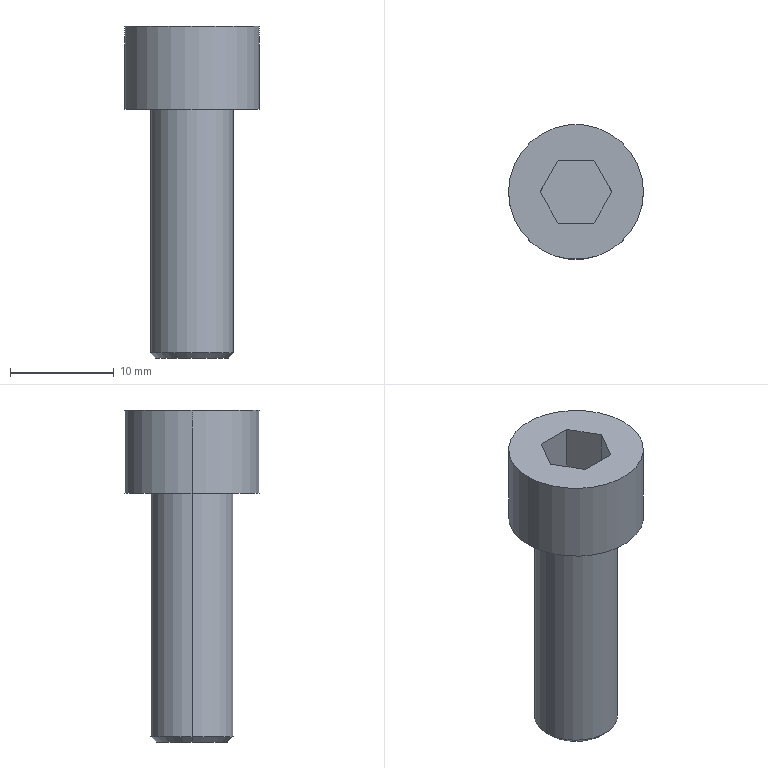Part | Creo | 1 solid | 16 faces | box 13 x 13 x 32 mm | volume 2101 mm3 | plane 10 | cylinder 4 | cone 2 | commonest cylinder face diameters 8 x2 13 x2
STEP:
#1=CARTESIAN_POINT('',(0.,0.,0.));
#2=DIRECTION('',(0.,0.,1.));
#3=DIRECTION('',(1.,0.,0.));
#4=AXIS2_PLACEMENT_3D('',#1,#2,#3);
#5=CARTESIAN_POINT('',(382.148,-184.728,-64.336));
#6=VERTEX_POINT('',#5);
#7=CARTESIAN_POINT('',(390.148,-184.728,-64.336));
#8=VERTEX_POINT('',#7);
#9=CARTESIAN_POINT('',(386.148,-184.728,-64.336));
#10=DIRECTION('',(0.,0.,-1.));
#11=DIRECTION('',(-1.,0.,0.));
#12=AXIS2_PLACEMENT_3D('',#9,#10,#11);
#13=CIRCLE('',#12,4.);
#14=EDGE_CURVE('',#6,#8,#13,.T.);
#15=ORIENTED_EDGE('',*,*,#14,.T.);
#16=CARTESIAN_POINT('',(390.148,-184.728,-40.844));
#17=VERTEX_POINT('',#16);
#18=CARTESIAN_POINT('',(390.148,-184.728,-40.844));
#19=DIRECTION('',(0.,0.,-1.));
#20=VECTOR('',#19,23.493);
#21=LINE('',#18,#20);
#22=EDGE_CURVE('',#17,#8,#21,.T.);
#23=ORIENTED_EDGE('',*,*,#22,.F.);
#24=CARTESIAN_POINT('',(382.148,-184.728,-40.844));
#25=VERTEX_POINT('',#24);
#26=CARTESIAN_POINT('',(386.148,-184.728,-40.844));
#27=DIRECTION('',(0.,0.,1.));
#28=DIRECTION('',(1.,0.,0.));
#29=AXIS2_PLACEMENT_3D('',#26,#27,#28);
#30=CIRCLE('',#29,4.);
#31=EDGE_CURVE('',#17,#25,#30,.T.);
#32=ORIENTED_EDGE('',*,*,#31,.T.);
#33=CARTESIAN_POINT('',(382.148,-184.728,-40.844));
#34=DIRECTION('',(0.,0.,-1.));
#35=VECTOR('',#34,23.493);
#36=LINE('',#33,#35);
#37=EDGE_CURVE('',#25,#6,#36,.T.);
#38=ORIENTED_EDGE('',*,*,#37,.T.);
#39=EDGE_LOOP('',(#15,#23,#32,#38));
#40=FACE_OUTER_BOUND('',#39,.F.);
#41=CARTESIAN_POINT('',(386.148,-184.728,-40.844));
#42=DIRECTION('',(0.,0.,-1.));
#43=DIRECTION('',(-1.,0.,0.));
#44=AXIS2_PLACEMENT_3D('',#41,#42,#43);
#45=CYLINDRICAL_SURFACE('',#44,4.);
#46=ADVANCED_FACE('',(#40),#45,.T.);
#47=CARTESIAN_POINT('',(382.656,-184.728,-64.844));
#48=VERTEX_POINT('',#47);
#49=CARTESIAN_POINT('',(389.641,-184.728,-64.844));
#50=VERTEX_POINT('',#49);
#51=CARTESIAN_POINT('',(386.148,-184.728,-64.844));
#52=DIRECTION('',(0.,0.,-1.));
#53=DIRECTION('',(-1.,0.,0.));
#54=AXIS2_PLACEMENT_3D('',#51,#52,#53);
#55=CIRCLE('',#54,3.493);
#56=EDGE_CURVE('',#48,#50,#55,.T.);
#57=ORIENTED_EDGE('',*,*,#56,.T.);
#58=CARTESIAN_POINT('',(389.641,-184.728,-64.844));
#59=DIRECTION('',(0.7071,0.,0.7071));
#60=VECTOR('',#59,0.7176);
#61=LINE('',#58,#60);
#62=EDGE_CURVE('',#50,#8,#61,.T.);
#63=ORIENTED_EDGE('',*,*,#62,.T.);
#64=ORIENTED_EDGE('',*,*,#14,.F.);
#65=CARTESIAN_POINT('',(382.656,-184.728,-64.844));
#66=DIRECTION('',(-0.7071,0.,0.7071));
#67=VECTOR('',#66,0.7176);
#68=LINE('',#65,#67);
#69=EDGE_CURVE('',#48,#6,#68,.T.);
#70=ORIENTED_EDGE('',*,*,#69,.F.);
#71=EDGE_LOOP('',(#57,#63,#64,#70));
#72=FACE_OUTER_BOUND('',#71,.F.);
#73=CARTESIAN_POINT('',(386.148,-184.728,-64.59));
#74=DIRECTION('',(0.,0.,1.));
#75=DIRECTION('',(1.,0.,0.));
#76=AXIS2_PLACEMENT_3D('',#73,#74,#75);
#77=CONICAL_SURFACE('',#76,3.746,45.);
#78=ADVANCED_FACE('',(#72),#77,.T.);
#79=ORIENTED_EDGE('',*,*,#56,.F.);
#80=CARTESIAN_POINT('',(386.148,-184.728,-64.844));
#81=DIRECTION('',(0.,0.,-1.));
#82=DIRECTION('',(1.,0.,0.));
#83=AXIS2_PLACEMENT_3D('',#80,#81,#82);
#84=CIRCLE('',#83,3.493);
#85=EDGE_CURVE('',#50,#48,#84,.T.);
#86=ORIENTED_EDGE('',*,*,#85,.F.);
#87=EDGE_LOOP('',(#79,#86));
#88=FACE_OUTER_BOUND('',#87,.F.);
#89=CARTESIAN_POINT('',(386.148,-184.728,-64.844));
#90=DIRECTION('',(0.,0.,1.));
#91=DIRECTION('',(1.,0.,0.));
#92=AXIS2_PLACEMENT_3D('',#89,#90,#91);
#93=PLANE('',#92);
#94=ADVANCED_FACE('',(#88),#93,.F.);
#95=ORIENTED_EDGE('',*,*,#85,.T.);
#96=ORIENTED_EDGE('',*,*,#69,.T.);
#97=CARTESIAN_POINT('',(386.148,-184.728,-64.336));
#98=DIRECTION('',(0.,0.,-1.));
#99=DIRECTION('',(1.,0.,0.));
#100=AXIS2_PLACEMENT_3D('',#97,#98,#99);
#101=CIRCLE('',#100,4.);
#102=EDGE_CURVE('',#8,#6,#101,.T.);
#103=ORIENTED_EDGE('',*,*,#102,.F.);
#104=ORIENTED_EDGE('',*,*,#62,.F.);
#105=EDGE_LOOP('',(#95,#96,#103,#104));
#106=FACE_OUTER_BOUND('',#105,.F.);
#107=CARTESIAN_POINT('',(386.148,-184.728,-64.59));
#108=DIRECTION('',(0.,0.,1.));
#109=DIRECTION('',(1.,0.,0.));
#110=AXIS2_PLACEMENT_3D('',#107,#108,#109);
#111=CONICAL_SURFACE('',#110,3.746,45.);
#112=ADVANCED_FACE('',(#106),#111,.T.);
#113=ORIENTED_EDGE('',*,*,#102,.T.);
#114=ORIENTED_EDGE('',*,*,#37,.F.);
#115=CARTESIAN_POINT('',(386.148,-184.728,-40.844));
#116=DIRECTION('',(0.,0.,1.));
#117=DIRECTION('',(-1.,0.,0.));
#118=AXIS2_PLACEMENT_3D('',#115,#116,#117);
#119=CIRCLE('',#118,4.);
#120=EDGE_CURVE('',#25,#17,#119,.T.);
#121=ORIENTED_EDGE('',*,*,#120,.T.);
#122=ORIENTED_EDGE('',*,*,#22,.T.);
#123=EDGE_LOOP('',(#113,#114,#121,#122));
#124=FACE_OUTER_BOUND('',#123,.F.);
#125=CARTESIAN_POINT('',(386.148,-184.728,-40.844));
#126=DIRECTION('',(0.,0.,-1.));
#127=DIRECTION('',(-1.,0.,0.));
#128=AXIS2_PLACEMENT_3D('',#125,#126,#127);
#129=CYLINDRICAL_SURFACE('',#128,4.);
#130=ADVANCED_FACE('',(#124),#129,.T.);
#131=CARTESIAN_POINT('',(379.648,-184.728,-40.844));
#132=VERTEX_POINT('',#131);
#133=CARTESIAN_POINT('',(392.648,-184.728,-40.844));
#134=VERTEX_POINT('',#133);
#135=CARTESIAN_POINT('',(386.148,-184.728,-40.844));
#136=DIRECTION('',(0.,0.,-1.));
#137=DIRECTION('',(-1.,0.,0.));
#138=AXIS2_PLACEMENT_3D('',#135,#136,#137);
#139=CIRCLE('',#138,6.5);
#140=EDGE_CURVE('',#132,#134,#139,.T.);
#141=ORIENTED_EDGE('',*,*,#140,.F.);
#142=CARTESIAN_POINT('',(386.148,-184.728,-40.844));
#143=DIRECTION('',(0.,0.,-1.));
#144=DIRECTION('',(1.,0.,0.));
#145=AXIS2_PLACEMENT_3D('',#142,#143,#144);
#146=CIRCLE('',#145,6.5);
#147=EDGE_CURVE('',#134,#132,#146,.T.);
#148=ORIENTED_EDGE('',*,*,#147,.F.);
#149=EDGE_LOOP('',(#141,#148));
#150=FACE_OUTER_BOUND('',#149,.F.);
#151=ORIENTED_EDGE('',*,*,#120,.F.);
#152=ORIENTED_EDGE('',*,*,#31,.F.);
#153=EDGE_LOOP('',(#151,#152));
#154=FACE_BOUND('',#153,.F.);
#155=CARTESIAN_POINT('',(386.148,-184.728,-40.844));
#156=DIRECTION('',(0.,0.,-1.));
#157=DIRECTION('',(-1.,0.,0.));
#158=AXIS2_PLACEMENT_3D('',#155,#156,#157);
#159=PLANE('',#158);
#160=ADVANCED_FACE('',(#150,#154),#159,.T.);
#161=CARTESIAN_POINT('',(392.648,-184.728,-32.844));
#162=VERTEX_POINT('',#161);
#163=CARTESIAN_POINT('',(379.648,-184.728,-32.844));
#164=VERTEX_POINT('',#163);
#165=CARTESIAN_POINT('',(386.148,-184.728,-32.844));
#166=DIRECTION('',(0.,0.,1.));
#167=DIRECTION('',(1.,0.,0.));
#168=AXIS2_PLACEMENT_3D('',#165,#166,#167);
#169=CIRCLE('',#168,6.5);
#170=EDGE_CURVE('',#162,#164,#169,.T.);
#171=ORIENTED_EDGE('',*,*,#170,.T.);
#172=CARTESIAN_POINT('',(379.648,-184.728,-40.844));
#173=DIRECTION('',(0.,0.,1.));
#174=VECTOR('',#173,8.);
#175=LINE('',#172,#174);
#176=EDGE_CURVE('',#132,#164,#175,.T.);
#177=ORIENTED_EDGE('',*,*,#176,.F.);
#178=ORIENTED_EDGE('',*,*,#140,.T.);
#179=CARTESIAN_POINT('',(392.648,-184.728,-40.844));
#180=DIRECTION('',(0.,0.,1.));
#181=VECTOR('',#180,8.);
#182=LINE('',#179,#181);
#183=EDGE_CURVE('',#134,#162,#182,.T.);
#184=ORIENTED_EDGE('',*,*,#183,.T.);
#185=EDGE_LOOP('',(#171,#177,#178,#184));
#186=FACE_OUTER_BOUND('',#185,.F.);
#187=CARTESIAN_POINT('',(386.148,-184.728,-40.844));
#188=DIRECTION('',(0.,0.,1.));
#189=DIRECTION('',(1.,0.,0.));
#190=AXIS2_PLACEMENT_3D('',#187,#188,#189);
#191=CYLINDRICAL_SURFACE('',#190,6.5);
#192=ADVANCED_FACE('',(#186),#191,.T.);
#193=CARTESIAN_POINT('',(386.148,-184.728,-32.844));
#194=DIRECTION('',(0.,0.,1.));
#195=DIRECTION('',(-1.,0.,0.));
#196=AXIS2_PLACEMENT_3D('',#193,#194,#195);
#197=CIRCLE('',#196,6.5);
#198=EDGE_CURVE('',#164,#162,#197,.T.);
#199=ORIENTED_EDGE('',*,*,#198,.F.);
#200=ORIENTED_EDGE('',*,*,#170,.F.);
#201=EDGE_LOOP('',(#199,#200));
#202=FACE_OUTER_BOUND('',#201,.F.);
#203=CARTESIAN_POINT('',(384.416,-181.728,-32.844));
#204=VERTEX_POINT('',#203);
#205=CARTESIAN_POINT('',(387.88,-181.728,-32.844));
#206=VERTEX_POINT('',#205);
#207=CARTESIAN_POINT('',(384.416,-181.728,-32.844));
#208=DIRECTION('',(1.,0.,0.));
#209=VECTOR('',#208,3.464);
#210=LINE('',#207,#209);
#211=EDGE_CURVE('',#204,#206,#210,.T.);
#212=ORIENTED_EDGE('',*,*,#211,.F.);
#213=CARTESIAN_POINT('',(382.684,-184.728,-32.844));
#214=VERTEX_POINT('',#213);
#215=CARTESIAN_POINT('',(382.684,-184.728,-32.844));
#216=DIRECTION('',(0.5,0.866,0.));
#217=VECTOR('',#216,3.464);
#218=LINE('',#215,#217);
#219=EDGE_CURVE('',#214,#204,#218,.T.);
#220=ORIENTED_EDGE('',*,*,#219,.F.);
#221=CARTESIAN_POINT('',(384.416,-187.728,-32.844));
#222=VERTEX_POINT('',#221);
#223=CARTESIAN_POINT('',(384.416,-187.728,-32.844));
#224=DIRECTION('',(-0.5,0.866,0.));
#225=VECTOR('',#224,3.464);
#226=LINE('',#223,#225);
#227=EDGE_CURVE('',#222,#214,#226,.T.);
#228=ORIENTED_EDGE('',*,*,#227,.F.);
#229=CARTESIAN_POINT('',(387.88,-187.728,-32.844));
#230=VERTEX_POINT('',#229);
#231=CARTESIAN_POINT('',(387.88,-187.728,-32.844));
#232=DIRECTION('',(-1.,0.,0.));
#233=VECTOR('',#232,3.464);
#234=LINE('',#231,#233);
#235=EDGE_CURVE('',#230,#222,#234,.T.);
#236=ORIENTED_EDGE('',*,*,#235,.F.);
#237=CARTESIAN_POINT('',(389.612,-184.728,-32.844));
#238=VERTEX_POINT('',#237);
#239=CARTESIAN_POINT('',(389.612,-184.728,-32.844));
#240=DIRECTION('',(-0.5,-0.866,0.));
#241=VECTOR('',#240,3.464);
#242=LINE('',#239,#241);
#243=EDGE_CURVE('',#238,#230,#242,.T.);
#244=ORIENTED_EDGE('',*,*,#243,.F.);
#245=CARTESIAN_POINT('',(387.88,-181.728,-32.844));
#246=DIRECTION('',(0.5,-0.866,0.));
#247=VECTOR('',#246,3.464);
#248=LINE('',#245,#247);
#249=EDGE_CURVE('',#206,#238,#248,.T.);
#250=ORIENTED_EDGE('',*,*,#249,.F.);
#251=EDGE_LOOP('',(#212,#220,#228,#236,#244,#250));
#252=FACE_BOUND('',#251,.F.);
#253=CARTESIAN_POINT('',(386.148,-184.728,-32.844));
#254=DIRECTION('',(0.,0.,1.));
#255=DIRECTION('',(1.,0.,0.));
#256=AXIS2_PLACEMENT_3D('',#253,#254,#255);
#257=PLANE('',#256);
#258=ADVANCED_FACE('',(#202,#252),#257,.T.);
#259=ORIENTED_EDGE('',*,*,#211,.T.);
#260=CARTESIAN_POINT('',(387.88,-181.728,-38.124));
#261=VERTEX_POINT('',#260);
#262=CARTESIAN_POINT('',(387.88,-181.728,-32.844));
#263=DIRECTION('',(0.,0.,-1.));
#264=VECTOR('',#263,5.28);
#265=LINE('',#262,#264);
#266=EDGE_CURVE('',#206,#261,#265,.T.);
#267=ORIENTED_EDGE('',*,*,#266,.T.);
#268=CARTESIAN_POINT('',(384.416,-181.728,-38.124));
#269=VERTEX_POINT('',#268);
#270=CARTESIAN_POINT('',(384.416,-181.728,-38.124));
#271=DIRECTION('',(1.,0.,0.));
#272=VECTOR('',#271,3.464);
#273=LINE('',#270,#272);
#274=EDGE_CURVE('',#269,#261,#273,.T.);
#275=ORIENTED_EDGE('',*,*,#274,.F.);
#276=CARTESIAN_POINT('',(384.416,-181.728,-32.844));
#277=DIRECTION('',(0.,0.,-1.));
#278=VECTOR('',#277,5.28);
#279=LINE('',#276,#278);
#280=EDGE_CURVE('',#204,#269,#279,.T.);
#281=ORIENTED_EDGE('',*,*,#280,.F.);
#282=EDGE_LOOP('',(#259,#267,#275,#281));
#283=FACE_OUTER_BOUND('',#282,.F.);
#284=CARTESIAN_POINT('',(387.88,-181.728,-38.124));
#285=DIRECTION('',(0.,1.,0.));
#286=DIRECTION('',(0.,0.,1.));
#287=AXIS2_PLACEMENT_3D('',#284,#285,#286);
#288=PLANE('',#287);
#289=ADVANCED_FACE('',(#283),#288,.F.);
#290=ORIENTED_EDGE('',*,*,#249,.T.);
#291=CARTESIAN_POINT('',(389.612,-184.728,-38.124));
#292=VERTEX_POINT('',#291);
#293=CARTESIAN_POINT('',(389.612,-184.728,-32.844));
#294=DIRECTION('',(0.,0.,-1.));
#295=VECTOR('',#294,5.28);
#296=LINE('',#293,#295);
#297=EDGE_CURVE('',#238,#292,#296,.T.);
#298=ORIENTED_EDGE('',*,*,#297,.T.);
#299=CARTESIAN_POINT('',(389.612,-184.728,-38.124));
#300=DIRECTION('',(-0.5,0.866,0.));
#301=VECTOR('',#300,3.464);
#302=LINE('',#299,#301);
#303=EDGE_CURVE('',#292,#261,#302,.T.);
#304=ORIENTED_EDGE('',*,*,#303,.T.);
#305=ORIENTED_EDGE('',*,*,#266,.F.);
#306=EDGE_LOOP('',(#290,#298,#304,#305));
#307=FACE_OUTER_BOUND('',#306,.F.);
#308=CARTESIAN_POINT('',(389.612,-184.728,-38.124));
#309=DIRECTION('',(0.866,0.5,0.));
#310=DIRECTION('',(-0.5,0.866,0.));
#311=AXIS2_PLACEMENT_3D('',#308,#309,#310);
#312=PLANE('',#311);
#313=ADVANCED_FACE('',(#307),#312,.F.);
#314=ORIENTED_EDGE('',*,*,#243,.T.);
#315=CARTESIAN_POINT('',(387.88,-187.728,-38.124));
#316=VERTEX_POINT('',#315);
#317=CARTESIAN_POINT('',(387.88,-187.728,-32.844));
#318=DIRECTION('',(0.,0.,-1.));
#319=VECTOR('',#318,5.28);
#320=LINE('',#317,#319);
#321=EDGE_CURVE('',#230,#316,#320,.T.);
#322=ORIENTED_EDGE('',*,*,#321,.T.);
#323=CARTESIAN_POINT('',(387.88,-187.728,-38.124));
#324=DIRECTION('',(0.5,0.866,0.));
#325=VECTOR('',#324,3.464);
#326=LINE('',#323,#325);
#327=EDGE_CURVE('',#316,#292,#326,.T.);
#328=ORIENTED_EDGE('',*,*,#327,.T.);
#329=ORIENTED_EDGE('',*,*,#297,.F.);
#330=EDGE_LOOP('',(#314,#322,#328,#329));
#331=FACE_OUTER_BOUND('',#330,.F.);
#332=CARTESIAN_POINT('',(387.88,-187.728,-38.124));
#333=DIRECTION('',(0.866,-0.5,0.));
#334=DIRECTION('',(0.5,0.866,0.));
#335=AXIS2_PLACEMENT_3D('',#332,#333,#334);
#336=PLANE('',#335);
#337=ADVANCED_FACE('',(#331),#336,.F.);
#338=ORIENTED_EDGE('',*,*,#235,.T.);
#339=CARTESIAN_POINT('',(384.416,-187.728,-38.124));
#340=VERTEX_POINT('',#339);
#341=CARTESIAN_POINT('',(384.416,-187.728,-32.844));
#342=DIRECTION('',(0.,0.,-1.));
#343=VECTOR('',#342,5.28);
#344=LINE('',#341,#343);
#345=EDGE_CURVE('',#222,#340,#344,.T.);
#346=ORIENTED_EDGE('',*,*,#345,.T.);
#347=CARTESIAN_POINT('',(387.88,-187.728,-38.124));
#348=DIRECTION('',(-1.,0.,0.));
#349=VECTOR('',#348,3.464);
#350=LINE('',#347,#349);
#351=EDGE_CURVE('',#316,#340,#350,.T.);
#352=ORIENTED_EDGE('',*,*,#351,.F.);
#353=ORIENTED_EDGE('',*,*,#321,.F.);
#354=EDGE_LOOP('',(#338,#346,#352,#353));
#355=FACE_OUTER_BOUND('',#354,.F.);
#356=CARTESIAN_POINT('',(384.416,-187.728,-38.124));
#357=DIRECTION('',(0.,-1.,0.));
#358=DIRECTION('',(0.,0.,-1.));
#359=AXIS2_PLACEMENT_3D('',#356,#357,#358);
#360=PLANE('',#359);
#361=ADVANCED_FACE('',(#355),#360,.F.);
#362=ORIENTED_EDGE('',*,*,#227,.T.);
#363=CARTESIAN_POINT('',(382.684,-184.728,-38.124));
#364=VERTEX_POINT('',#363);
#365=CARTESIAN_POINT('',(382.684,-184.728,-32.844));
#366=DIRECTION('',(0.,0.,-1.));
#367=VECTOR('',#366,5.28);
#368=LINE('',#365,#367);
#369=EDGE_CURVE('',#214,#364,#368,.T.);
#370=ORIENTED_EDGE('',*,*,#369,.T.);
#371=CARTESIAN_POINT('',(382.684,-184.728,-38.124));
#372=DIRECTION('',(0.5,-0.866,0.));
#373=VECTOR('',#372,3.464);
#374=LINE('',#371,#373);
#375=EDGE_CURVE('',#364,#340,#374,.T.);
#376=ORIENTED_EDGE('',*,*,#375,.T.);
#377=ORIENTED_EDGE('',*,*,#345,.F.);
#378=EDGE_LOOP('',(#362,#370,#376,#377));
#379=FACE_OUTER_BOUND('',#378,.F.);
#380=CARTESIAN_POINT('',(382.684,-184.728,-38.124));
#381=DIRECTION('',(-0.866,-0.5,0.));
#382=DIRECTION('',(0.5,-0.866,0.));
#383=AXIS2_PLACEMENT_3D('',#380,#381,#382);
#384=PLANE('',#383);
#385=ADVANCED_FACE('',(#379),#384,.F.);
#386=ORIENTED_EDGE('',*,*,#219,.T.);
#387=ORIENTED_EDGE('',*,*,#280,.T.);
#388=CARTESIAN_POINT('',(384.416,-181.728,-38.124));
#389=DIRECTION('',(-0.5,-0.866,0.));
#390=VECTOR('',#389,3.464);
#391=LINE('',#388,#390);
#392=EDGE_CURVE('',#269,#364,#391,.T.);
#393=ORIENTED_EDGE('',*,*,#392,.T.);
#394=ORIENTED_EDGE('',*,*,#369,.F.);
#395=EDGE_LOOP('',(#386,#387,#393,#394));
#396=FACE_OUTER_BOUND('',#395,.F.);
#397=CARTESIAN_POINT('',(384.416,-181.728,-38.124));
#398=DIRECTION('',(-0.866,0.5,0.));
#399=DIRECTION('',(-0.5,-0.866,0.));
#400=AXIS2_PLACEMENT_3D('',#397,#398,#399);
#401=PLANE('',#400);
#402=ADVANCED_FACE('',(#396),#401,.F.);
#403=ORIENTED_EDGE('',*,*,#274,.T.);
#404=ORIENTED_EDGE('',*,*,#303,.F.);
#405=ORIENTED_EDGE('',*,*,#327,.F.);
#406=ORIENTED_EDGE('',*,*,#351,.T.);
#407=ORIENTED_EDGE('',*,*,#375,.F.);
#408=ORIENTED_EDGE('',*,*,#392,.F.);
#409=EDGE_LOOP('',(#403,#404,#405,#406,#407,#408));
#410=FACE_OUTER_BOUND('',#409,.F.);
#411=CARTESIAN_POINT('',(384.416,-181.728,-38.124));
#412=DIRECTION('',(0.,0.,1.));
#413=DIRECTION('',(1.,0.,0.));
#414=AXIS2_PLACEMENT_3D('',#411,#412,#413);
#415=PLANE('',#414);
#416=ADVANCED_FACE('',(#410),#415,.T.);
#417=ORIENTED_EDGE('',*,*,#198,.T.);
#418=ORIENTED_EDGE('',*,*,#183,.F.);
#419=ORIENTED_EDGE('',*,*,#147,.T.);
#420=ORIENTED_EDGE('',*,*,#176,.T.);
#421=EDGE_LOOP('',(#417,#418,#419,#420));
#422=FACE_OUTER_BOUND('',#421,.F.);
#423=CARTESIAN_POINT('',(386.148,-184.728,-40.844));
#424=DIRECTION('',(0.,0.,1.));
#425=DIRECTION('',(1.,0.,0.));
#426=AXIS2_PLACEMENT_3D('',#423,#424,#425);
#427=CYLINDRICAL_SURFACE('',#426,6.5);
#428=ADVANCED_FACE('',(#422),#427,.T.);
#429=CLOSED_SHELL('',(#46,#78,#94,#112,#130,#160,#192,#258,#289,#313,#337,#361,#385,#402,#416,#428));
#430=MANIFOLD_SOLID_BREP('',#429);
#431=(LENGTH_UNIT()NAMED_UNIT(*)SI_UNIT(.MILLI.,.METRE.));
#432=UNCERTAINTY_MEASURE_WITH_UNIT(LENGTH_MEASURE(0.00369),#431,'','');
#433=(NAMED_UNIT(*)PLANE_ANGLE_UNIT()SI_UNIT($,.RADIAN.));
#434=PLANE_ANGLE_MEASURE_WITH_UNIT(PLANE_ANGLE_MEASURE(0.01745),#433);
#435=(CONVERSION_BASED_UNIT('DEGREE',#434)NAMED_UNIT(*)PLANE_ANGLE_UNIT());
#436=(NAMED_UNIT(*)SI_UNIT($,.STERADIAN.)SOLID_ANGLE_UNIT());
#437=(GEOMETRIC_REPRESENTATION_CONTEXT(3)GLOBAL_UNCERTAINTY_ASSIGNED_CONTEXT((#432))GLOBAL_UNIT_ASSIGNED_CONTEXT((#431,#435,#436))REPRESENTATION_CONTEXT('',''));
#438=ADVANCED_BREP_SHAPE_REPRESENTATION('',(#4,#430),#437);